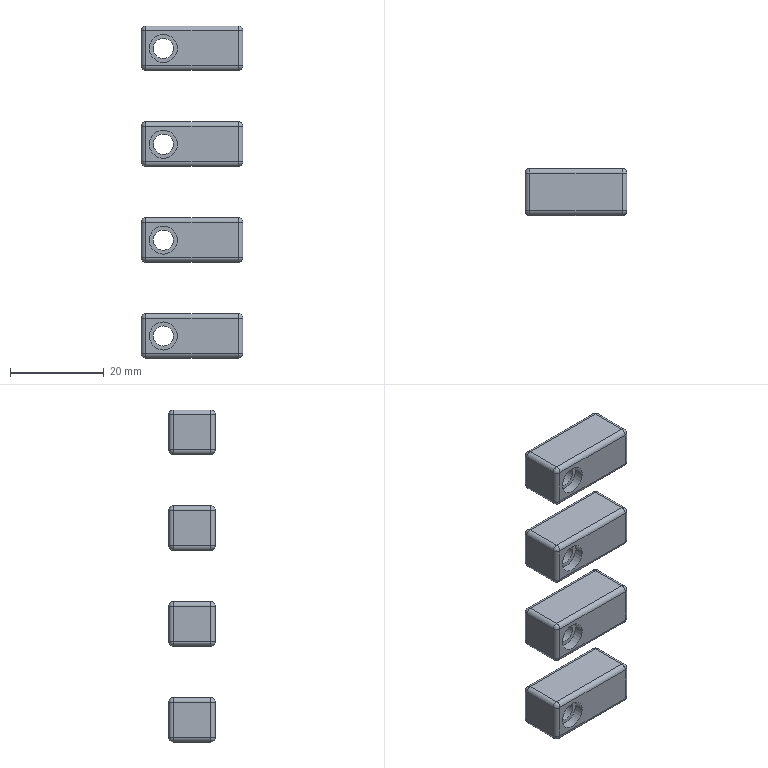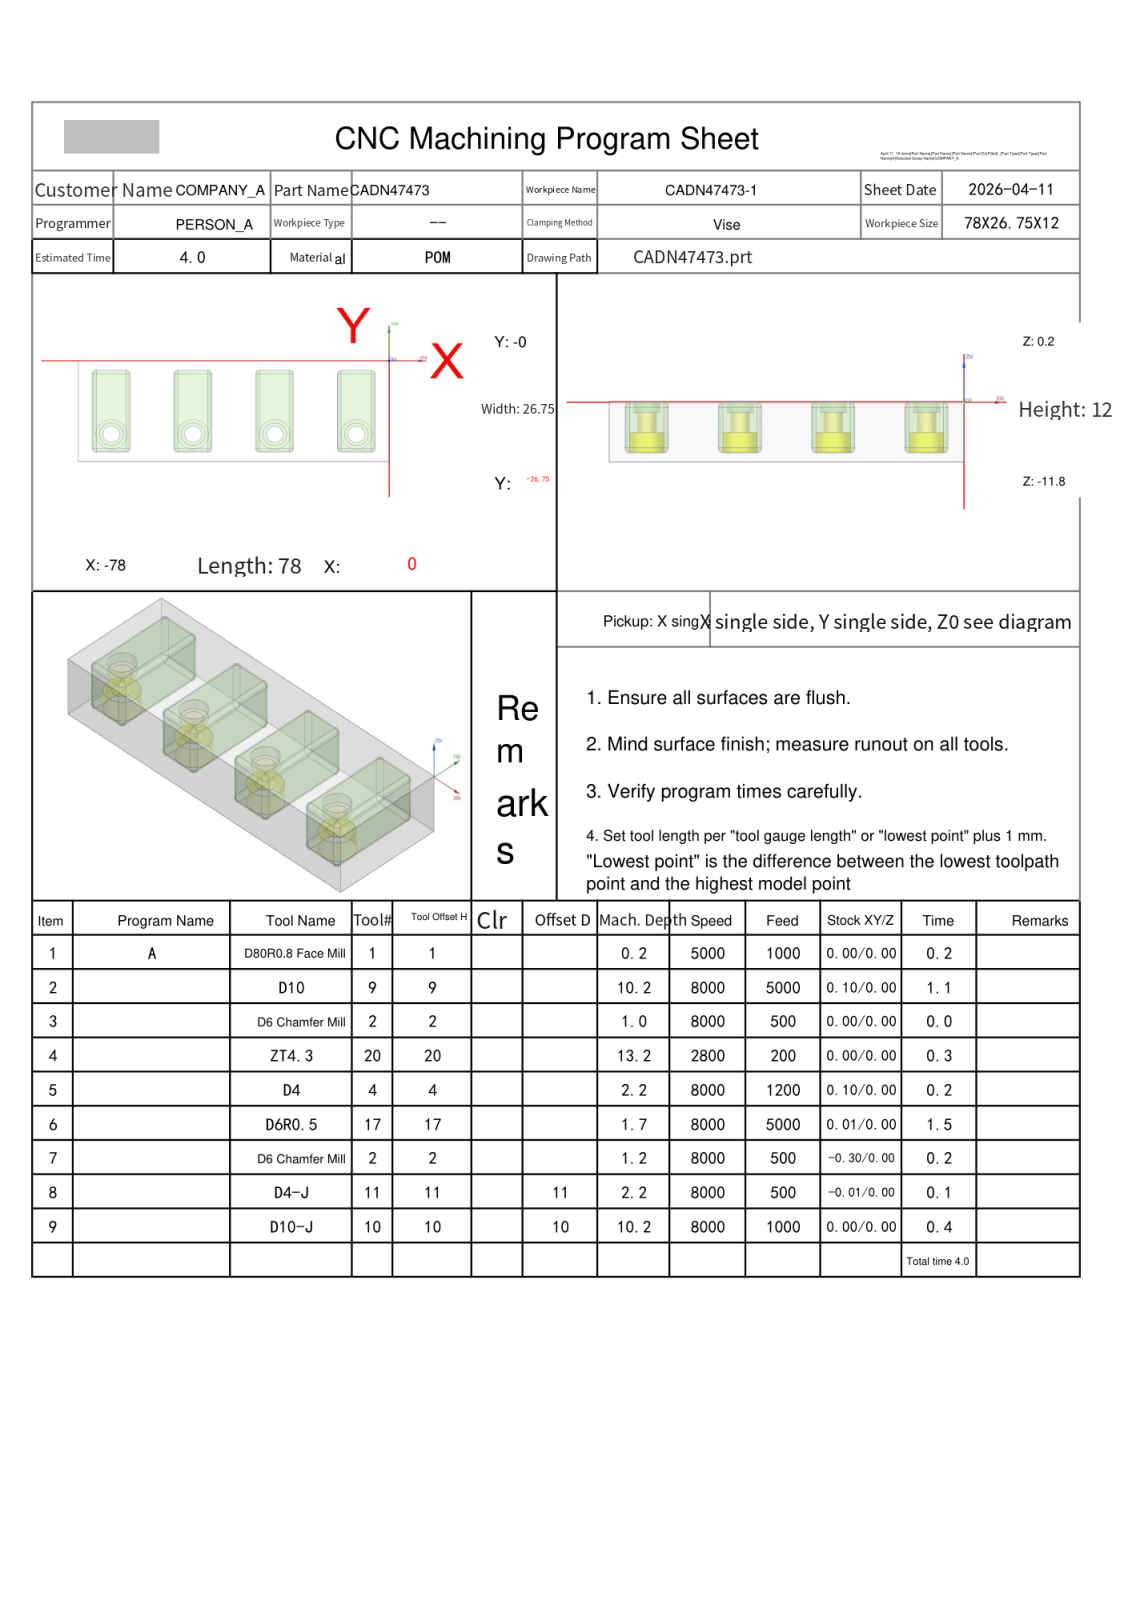NC program | NX | posted by the shop | part box 21.75 x 10 x 71 mm
Lines 15338 to 15665 of 15665:
N7 T02 M06
(D6 Chamfer Mill  D=6. R=0. H=02 ce=-0.30 di=0.00)
G00 G90 G54 X-7.034 Y-21.481 M03 S8000
G43 H02 Z20.
M08
Z2.5
G01 X-6.952 Y-21.433 Z2.465 F500.
X-6.691 Y-21.236 Z2.346
X-6.46 Y-21.004 Z2.227
X-6.264 Y-20.741 Z2.108
X-6.108 Y-20.454 Z1.989
X-5.993 Y-20.147 Z1.87
X-5.924 Y-19.827 Z1.75
X-5.901 Y-19.5 Z1.631
X-5.924 Y-19.173 Z1.512
X-5.993 Y-18.853 Z1.393
X-6.108 Y-18.546 Z1.274
X-6.264 Y-18.259 Z1.154
X-6.46 Y-17.996 Z1.035
X-6.691 Y-17.764 Z.916
X-6.952 Y-17.567 Z.797
X-7.156 Y-17.449 Z.711
X-7.457 Y-17.321 Z.592
X-7.774 Y-17.238 Z.473
X-8.099 Y-17.199 Z.354
X-8.426 Y-17.208 Z.235
X-8.749 Y-17.262 Z.115
X-9.061 Y-17.362 Z-.004
X-9.355 Y-17.506 Z-.123
X-9.627 Y-17.689 Z-.242
X-9.869 Y-17.909 Z-.361
X-10.078 Y-18.161 Z-.48
X-10.249 Y-18.441 Z-.6
X-10.378 Y-18.741 Z-.719
X-10.464 Y-19.057 Z-.838
X-10.504 Y-19.382 Z-.957
Y-19.5 Z-1.
G03 X-8.204 Y-21.8 I2.3 J0.0
X-5.904 Y-19.5 I0.0 J2.3
X-8.204 Y-17.2 I-2.3 J0.0
X-10.504 Y-19.5 I0.0 J-2.3
X-10.45 Y-19.996 I2.3 J0.0
G01 Z1.5
G00 Z20.
X-27.534 Y-21.481
Z2.5
G01 X-27.452 Y-21.433 Z2.465
X-27.191 Y-21.236 Z2.346
X-26.96 Y-21.004 Z2.227
X-26.764 Y-20.741 Z2.108
X-26.608 Y-20.454 Z1.989
X-26.493 Y-20.147 Z1.87
X-26.424 Y-19.827 Z1.75
X-26.401 Y-19.5 Z1.631
X-26.424 Y-19.173 Z1.512
X-26.493 Y-18.853 Z1.393
X-26.608 Y-18.546 Z1.274
X-26.764 Y-18.259 Z1.154
X-26.96 Y-17.996 Z1.035
X-27.191 Y-17.764 Z.916
X-27.452 Y-17.567 Z.797
X-27.656 Y-17.449 Z.711
X-27.957 Y-17.321 Z.592
X-28.274 Y-17.238 Z.473
X-28.599 Y-17.199 Z.354
X-28.926 Y-17.208 Z.235
X-29.249 Y-17.262 Z.115
X-29.561 Y-17.362 Z-.004
X-29.855 Y-17.506 Z-.123
X-30.127 Y-17.689 Z-.242
X-30.369 Y-17.909 Z-.361
X-30.578 Y-18.161 Z-.48
X-30.749 Y-18.441 Z-.6
X-30.878 Y-18.741 Z-.719
X-30.964 Y-19.057 Z-.838
X-31.004 Y-19.382 Z-.957
Y-19.5 Z-1.
G03 X-28.704 Y-21.8 I2.3 J0.0
X-26.404 Y-19.5 I0.0 J2.3
X-28.704 Y-17.2 I-2.3 J0.0
X-31.004 Y-19.5 I0.0 J-2.3
X-30.95 Y-19.996 I2.3 J0.0
G01 Z1.5
G00 Z20.
X-48.034 Y-21.481
Z2.5
G01 X-47.952 Y-21.433 Z2.465
X-47.691 Y-21.236 Z2.346
X-47.46 Y-21.004 Z2.227
X-47.264 Y-20.741 Z2.108
X-47.108 Y-20.454 Z1.989
X-46.993 Y-20.147 Z1.87
X-46.924 Y-19.827 Z1.75
X-46.901 Y-19.5 Z1.631
X-46.924 Y-19.173 Z1.512
X-46.993 Y-18.853 Z1.393
X-47.108 Y-18.546 Z1.274
X-47.264 Y-18.259 Z1.154
X-47.46 Y-17.996 Z1.035
X-47.691 Y-17.764 Z.916
X-47.952 Y-17.567 Z.797
X-48.156 Y-17.449 Z.711
X-48.457 Y-17.321 Z.592
X-48.774 Y-17.238 Z.473
X-49.099 Y-17.199 Z.354
X-49.426 Y-17.208 Z.235
X-49.749 Y-17.262 Z.115
X-50.061 Y-17.362 Z-.004
X-50.355 Y-17.506 Z-.123
X-50.627 Y-17.689 Z-.242
X-50.869 Y-17.909 Z-.361
X-51.078 Y-18.161 Z-.48
X-51.249 Y-18.441 Z-.6
X-51.378 Y-18.741 Z-.719
X-51.464 Y-19.057 Z-.838
X-51.504 Y-19.382 Z-.957
Y-19.5 Z-1.
G03 X-49.204 Y-21.8 I2.3 J0.0
X-46.904 Y-19.5 I0.0 J2.3
X-49.204 Y-17.2 I-2.3 J0.0
X-51.504 Y-19.5 I0.0 J-2.3
X-51.45 Y-19.996 I2.3 J0.0
G01 Z1.5
G00 Z20.
X-68.534 Y-21.481
Z2.5
G01 X-68.452 Y-21.433 Z2.465
X-68.191 Y-21.236 Z2.346
X-67.96 Y-21.004 Z2.227
X-67.764 Y-20.741 Z2.108
X-67.608 Y-20.454 Z1.989
X-67.493 Y-20.147 Z1.87
X-67.424 Y-19.827 Z1.75
X-67.401 Y-19.5 Z1.631
X-67.424 Y-19.173 Z1.512
X-67.493 Y-18.853 Z1.393
X-67.608 Y-18.546 Z1.274
X-67.764 Y-18.259 Z1.154
X-67.96 Y-17.996 Z1.035
X-68.191 Y-17.764 Z.916
X-68.452 Y-17.567 Z.797
X-68.656 Y-17.449 Z.711
X-68.957 Y-17.321 Z.592
X-69.274 Y-17.238 Z.473
X-69.599 Y-17.199 Z.354
X-69.926 Y-17.208 Z.235
X-70.249 Y-17.262 Z.115
X-70.561 Y-17.362 Z-.004
X-70.855 Y-17.506 Z-.123
X-71.127 Y-17.689 Z-.242
X-71.369 Y-17.909 Z-.361
X-71.578 Y-18.161 Z-.48
X-71.749 Y-18.441 Z-.6
X-71.878 Y-18.741 Z-.719
X-71.964 Y-19.057 Z-.838
X-72.004 Y-19.382 Z-.957
Y-19.5 Z-1.
G03 X-69.704 Y-21.8 I2.3 J0.0
X-67.404 Y-19.5 I0.0 J2.3
X-69.704 Y-17.2 I-2.3 J0.0
X-72.004 Y-19.5 I0.0 J-2.3
X-71.95 Y-19.996 I2.3 J0.0
G01 Z1.5
G00 Z20.
G91 G28 Z0.0
M05
M09
G91 G28 Z0.0
M01
N8 T11 M06
(D4-J  D=4. R=0. H=11 ce=-0.01 di=0.00)
G00 G90 G54 X-8.148 Y-19.708 M03 S8000
G43 H11 Z10.2
M08
Z-1.
G01 Z-2. F500.
G41 D11
X-7.989 Y-20.3
G03 X-7.189 Y-19.5 I0.0 J.8
X-8.204 Y-18.485 I-1.015 J0.0
X-9.219 Y-19.5 I0.0 J-1.015
X-8.204 Y-20.515 I1.015 J0.0
X-7.189 Y-19.5 I0.0 J1.015
X-7.267 Y-19.11 I-1.015 J0.0
X-8.005 Y-18.617 I-.739 J-.307
X-8.313 Y-18.679 I0.0 J-.8
G01 G40 X-8.232 Y-19.287
Z-1.
G00 Z10.2
X-28.911 Y-19.556
Z-1.
G01 Z-2.
G41 D11
X-29.504 Y-19.715
G03 X-28.704 Y-20.515 I.8 J0.0
X-27.689 Y-19.5 I0.0 J1.015
X-28.704 Y-18.485 I-1.015 J0.0
X-29.719 Y-19.5 I0.0 J-1.015
X-28.704 Y-20.515 I1.015 J0.0
X-28.314 Y-20.437 I0.0 J1.015
X-27.821 Y-19.699 I-.307 J.739
X-27.883 Y-19.391 I-.8 J0.0
G01 G40 X-28.491 Y-19.472
Z-1.
G00 Z10.2
X-49.411 Y-19.556
Z-1.
G01 Z-2.
G41 D11
X-50.004 Y-19.715
G03 X-49.204 Y-20.515 I.8 J0.0
X-48.189 Y-19.5 I0.0 J1.015
X-49.204 Y-18.485 I-1.015 J0.0
X-50.219 Y-19.5 I0.0 J-1.015
X-49.204 Y-20.515 I1.015 J0.0
X-48.814 Y-20.437 I0.0 J1.015
X-48.321 Y-19.699 I-.307 J.739
X-48.383 Y-19.391 I-.8 J0.0
G01 G40 X-48.991 Y-19.472
Z-1.
G00 Z10.2
X-69.911 Y-19.556
Z-1.
G01 Z-2.
G41 D11
X-70.504 Y-19.715
G03 X-69.704 Y-20.515 I.8 J0.0
X-68.689 Y-19.5 I0.0 J1.015
X-69.704 Y-18.485 I-1.015 J0.0
X-70.719 Y-19.5 I0.0 J-1.015
X-69.704 Y-20.515 I1.015 J0.0
X-69.314 Y-20.437 I0.0 J1.015
X-68.821 Y-19.699 I-.307 J.739
X-68.883 Y-19.391 I-.8 J0.0
G01 G40 X-69.491 Y-19.472
Z-1.
G00 Z10.2
G91 G28 Z0.0
M05
M09
G91 G28 Z0.0
M01
N9 T10 M06
(D10-J  D=10. R=0. H=10 ce=0.00 di=0.00)
G00 G90 G54 X-18.56 Y-.711 M03 S8000
G43 H10 Z20.
M08
Z-9.5
G01 Z-10. F1000.
G41 D10
X-18. Y-2.5
G03 X-19. Y-3.5 I0.0 J-1.
G01 Y-23.25
G02 X-25. Y-29.25 I-6. J0.0
G01 X-32.5
G02 X-38.5 Y-23.25 I0.0 J6.
G01 Y-3.5
G02 X-32.5 Y2.5 I6. J0.0
G01 X-25.
G02 X-19. Y-3.5 I0.0 J-6.
G01 Y-4.
G03 X-18. Y-5. I1. J0.0
G01 G40 Y-4.8
X-19. Y-4.3
G41 D10
Y-4.5
G03 X-18. Y-3.5 I0.0 J1.
G02 X-12. Y2.5 I6. J0.0
G01 X-4.5
G02 X1.5 Y-3.5 I0.0 J-6.
G01 Y-23.25
G02 X-4.5 Y-29.25 I-6. J0.0
G01 X-12.
G02 X-18. Y-23.25 I0.0 J6.
G01 Y-3.5
G02 X-17.979 Y-3.001 I6. J0.0
G01 X-17.976 Y-2.917
G03 X-18.892 Y-1.921 I-1. J0.0
G01 X-18.5 Y-.902
G40 X-18.428 Y-.715
Z-9.5
G00 Z20.
X-50.25 Y3.7
Z-9.5
G01 Z-10.
G41 D10
Y3.5
G03 X-49.25 Y2.5 I1. J0.0
G01 X-45.5
G02 X-39.5 Y-3.5 I0.0 J-6.
G01 Y-23.25
G02 X-45.5 Y-29.25 I-6. J0.0
G01 X-53.
G02 X-59. Y-23.25 I0.0 J6.
G01 Y-3.5
G02 X-53. Y2.5 I6. J0.0
G01 X-49.25
X-48.75
G03 X-47.75 Y3.5 I0.0 J1.
G01 G40 Y3.7
Z-9.5
G00 Z20.
X-80.7 Y-14.375
Z-9.5
G01 Z-10.
G41 D10
X-80.5
G03 X-79.5 Y-13.375 I0.0 J1.
G01 Y-3.5
G02 X-73.5 Y2.5 I6. J0.0
G01 X-66.
G02 X-60. Y-3.5 I0.0 J-6.
G01 Y-23.25
G02 X-66. Y-29.25 I-6. J0.0
G01 X-73.5
G02 X-79.5 Y-23.25 I0.0 J6.
G01 Y-13.375
Y-12.875
G03 X-80.5 Y-11.875 I-1. J0.0
G01 G40 X-80.7
Z-9.5
G00 Z20.
M05
M09
G91 G28 Z0.0
G91 G28 Y0.0
M30
%